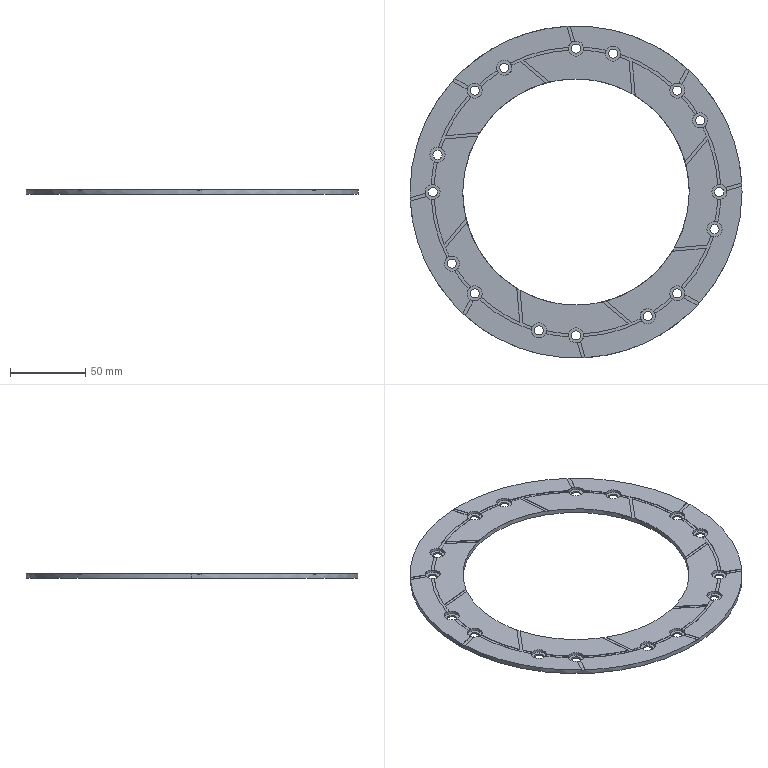Part | SolidWorks | features ICE 3, Extrusion 1 | 1 solid | 197 faces | box 220 x 220 x 3 mm | volume 57628 mm3 | cylinder 108 | plane 89 | commonest cylinder face diameters 6 x32 10 x32 188 x24 192 x16 150 x2 220 x2